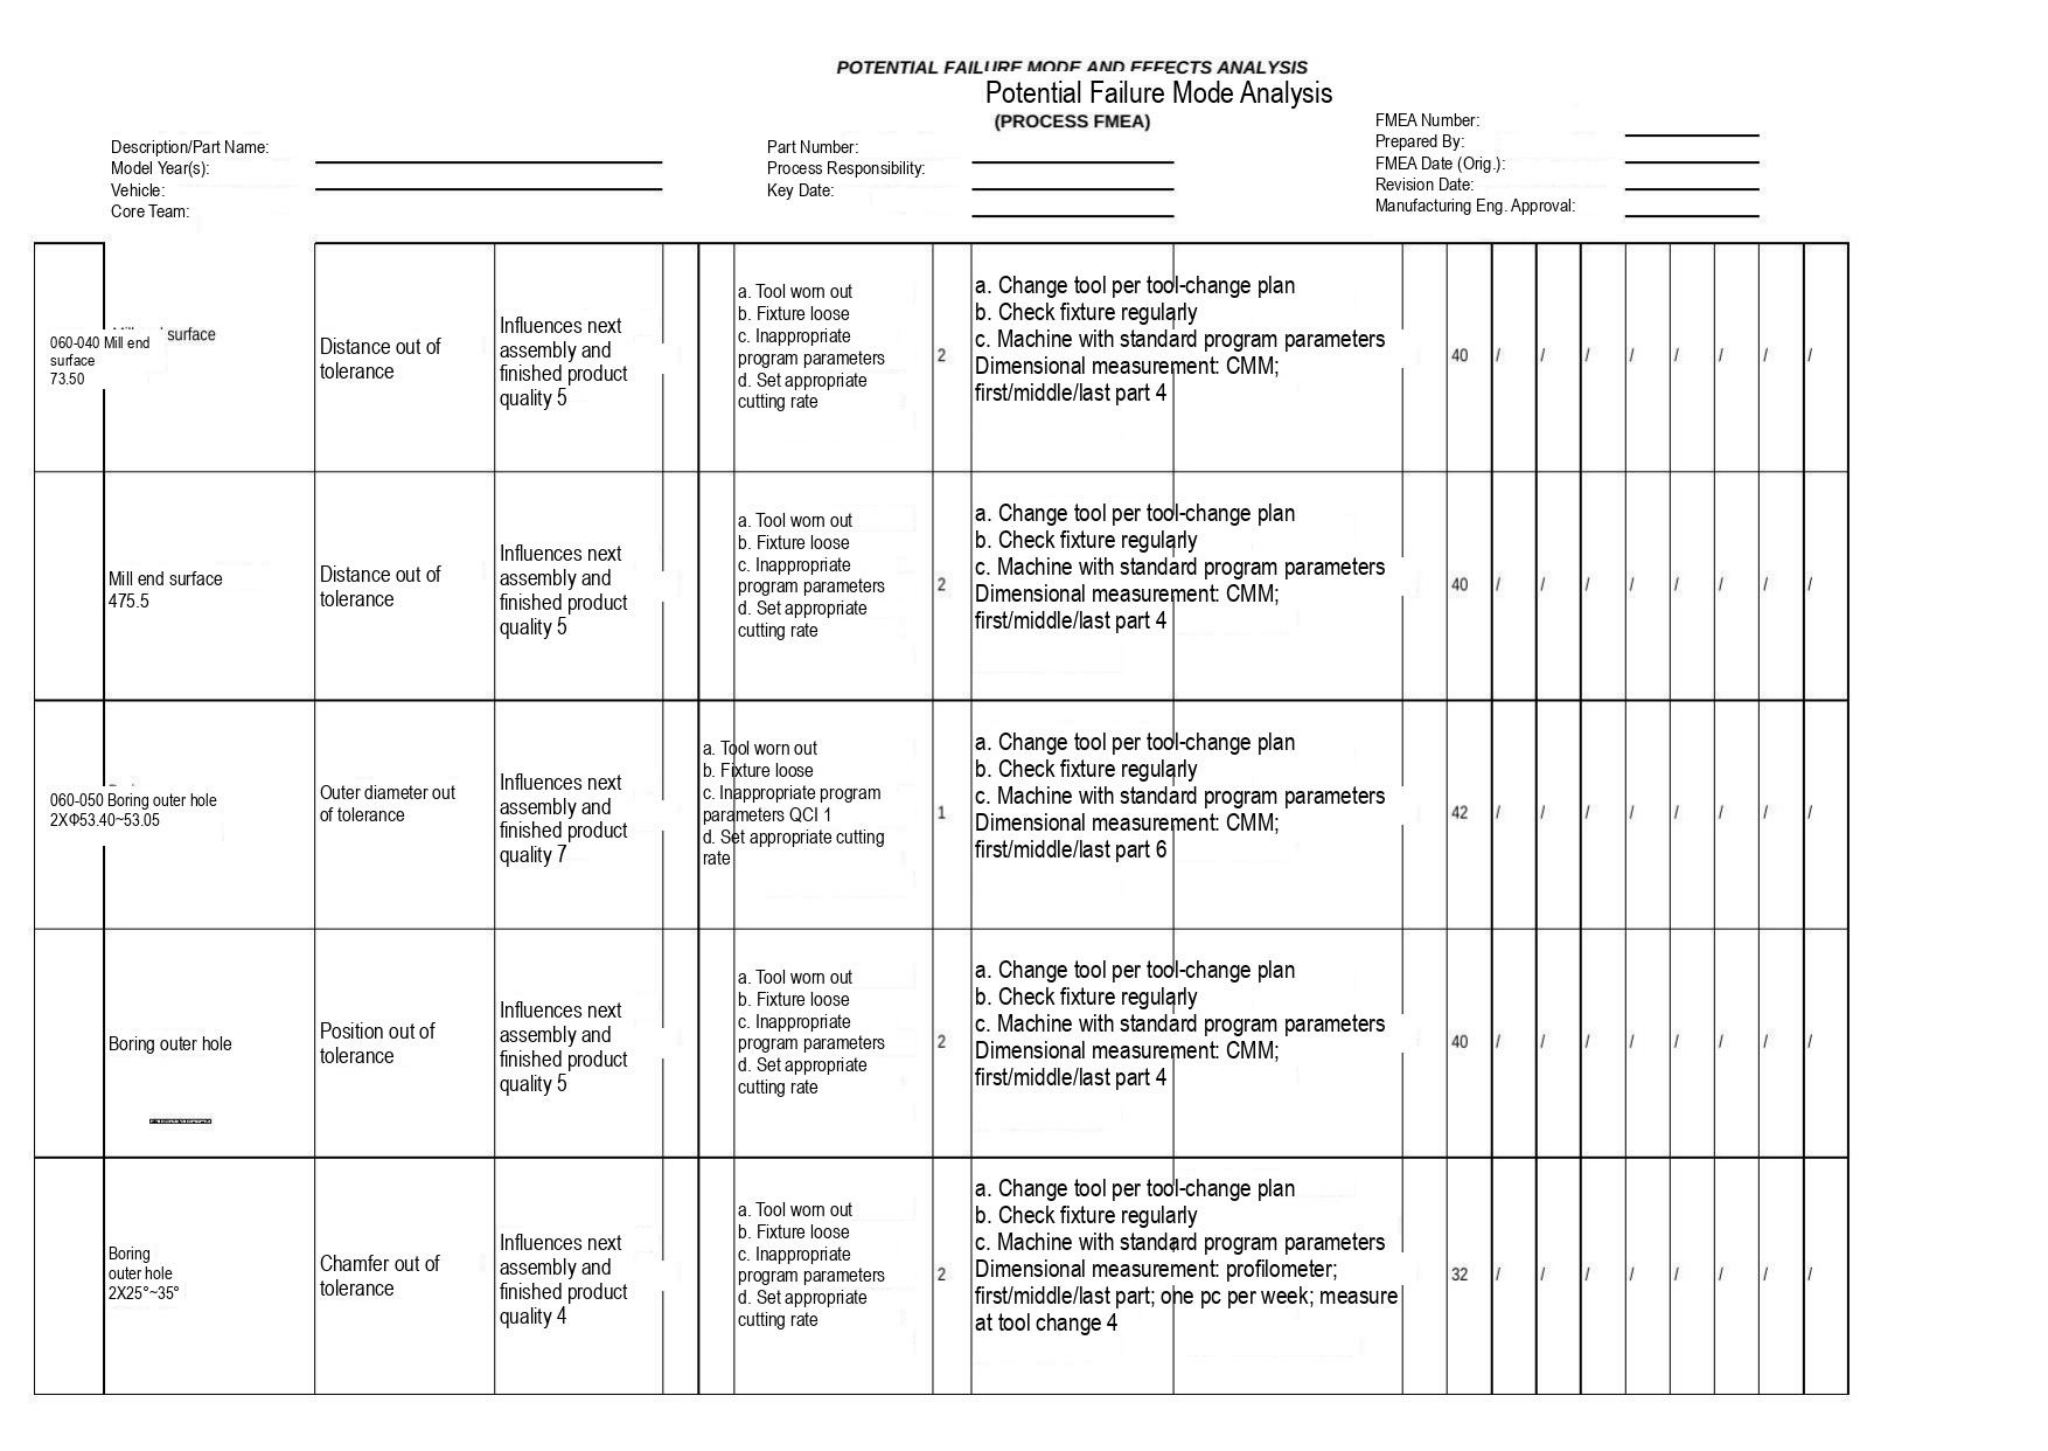**POTENTIAL FAILURE MODE AND EFFECTS ANALYSIS**

Potential Failure Mode Analysis

**(PROCESS FMEA)**

Description/Part Name:
Model Year(s):
Vehicle:
Core Team:

Part Number:
Process Responsibility:
Key Date:

FMEA Number:
Prepared By:
FMEA Date (Orig.):
Revision Date:
Manufacturing Eng. Approval:

| | | | | | | | | | | | | | | | | | | | |
|---|---|---|---|---|---|---|---|---|---|---|---|---|---|---|---|---|---|---|---|
| 060-040 Mill end surface 73.50 | surface | Distance out of tolerance | Influences next assembly and finished product quality 5 | | | a. Tool worn out<br>b. Fixture loose<br>c. Inappropriate program parameters<br>d. Set appropriate cutting rate | 2 | a. Change tool per tool-change plan<br>b. Check fixture regularly<br>c. Machine with standard program parameters<br>Dimensional measurement: CMM; first/middle/last part 4 | | | 40 | / | / | / | / | / | / | / | / |
| | Mill end surface 475.5 | Distance out of tolerance | Influences next assembly and finished product quality 5 | | | a. Tool worn out<br>b. Fixture loose<br>c. Inappropriate program parameters<br>d. Set appropriate cutting rate | 2 | a. Change tool per tool-change plan<br>b. Check fixture regularly<br>c. Machine with standard program parameters<br>Dimensional measurement: CMM; first/middle/last part 4 | | | 40 | / | / | / | / | / | / | / | / |
| 060-050 Boring outer hole 2XΦ53.40~53.05 | | Outer diameter out of tolerance | Influences next assembly and finished product quality 7 | | a. Tool worn out<br>b. Fixture loose<br>c. Inappropriate program parameters QCI 1<br>d. Set appropriate cutting rate | | 1 | a. Change tool per tool-change plan<br>b. Check fixture regularly<br>c. Machine with standard program parameters<br>Dimensional measurement: CMM; first/middle/last part 6 | | | 42 | / | / | / | / | / | / | / | / |
| | Boring outer hole | Position out of tolerance | Influences next assembly and finished product quality 5 | | | a. Tool worn out<br>b. Fixture loose<br>c. Inappropriate program parameters<br>d. Set appropriate cutting rate | 2 | a. Change tool per tool-change plan<br>b. Check fixture regularly<br>c. Machine with standard program parameters<br>Dimensional measurement: CMM; first/middle/last part 4 | | | 40 | / | / | / | / | / | / | / | / |
| | Boring outer hole 2X25°~35° | Chamfer out of tolerance | Influences next assembly and finished product quality 4 | | | a. Tool worn out<br>b. Fixture loose<br>c. Inappropriate program parameters<br>d. Set appropriate cutting rate | 2 | a. Change tool per tool-change plan<br>b. Check fixture regularly<br>c. Machine with standard program parameters<br>Dimensional measurement: profilometer; first/middle/last part; one pc per week; measure at tool change 4 | | | 32 | / | / | / | / | / | / | / | / |
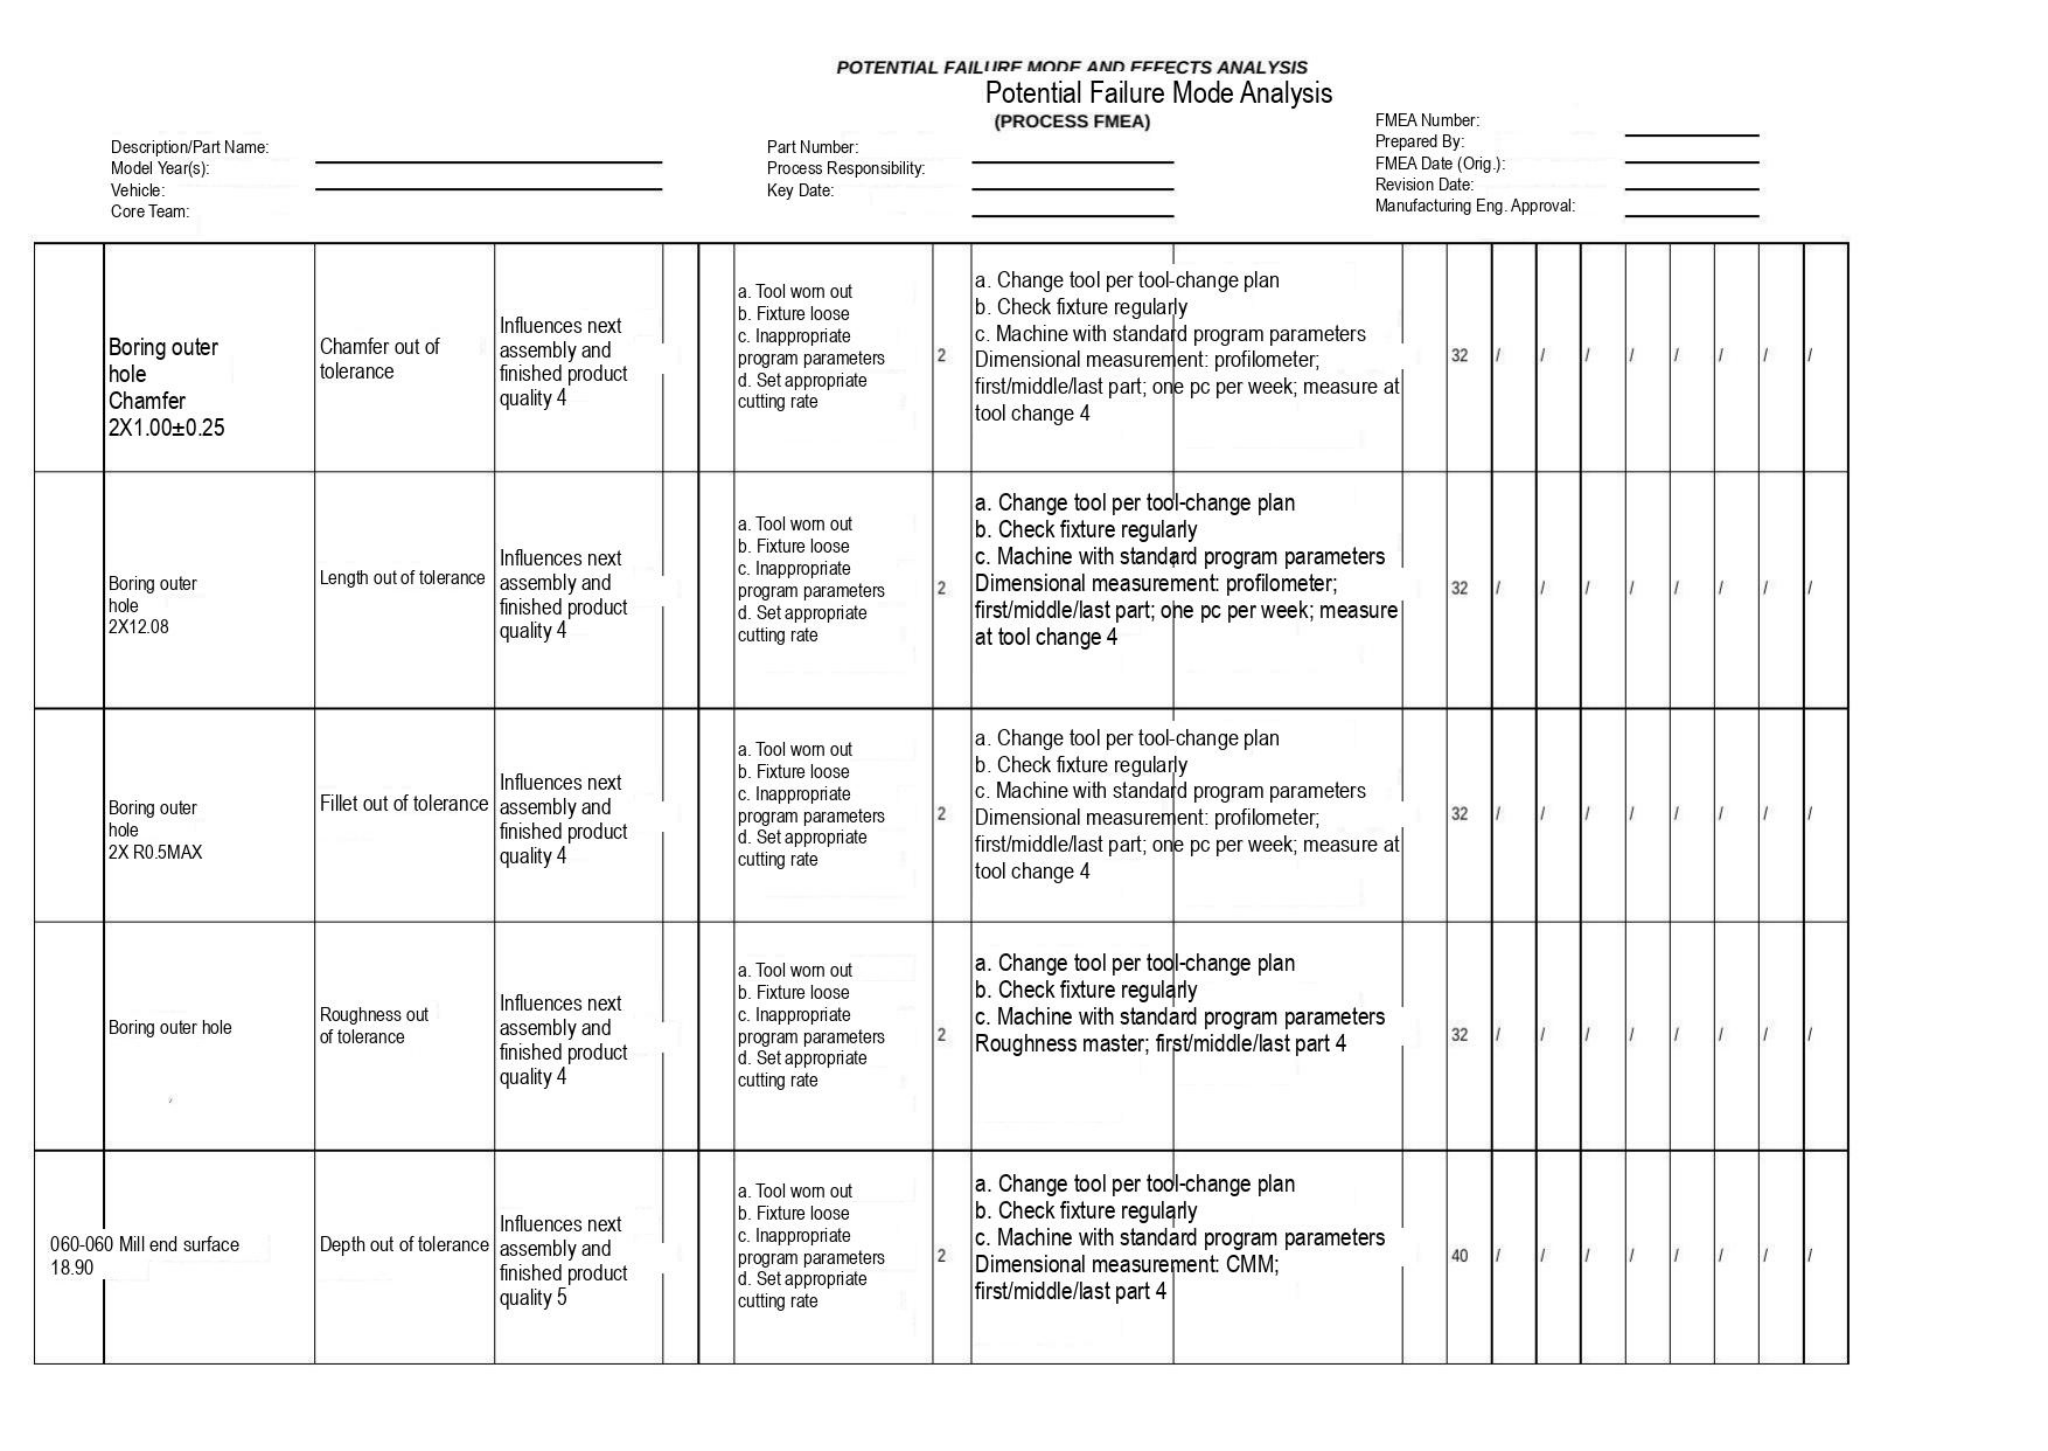POTENTIAL FAILURE MODE AND EFFECTS ANALYSIS

Potential Failure Mode Analysis

(PROCESS FMEA)

Description/Part Name:
Model Year(s):
Vehicle:
Core Team:

Part Number:
Process Responsibility:
Key Date:

FMEA Number:
Prepared By:
FMEA Date (Orig.):
Revision Date:
Manufacturing Eng. Approval:

| | | | | | | | | | | | | | | | | | | |
|---|---|---|---|---|---|---|---|---|---|---|---|---|---|---|---|---|---|---|
| | Boring outer hole Chamfer 2X1.00±0.25 | Chamfer out of tolerance | Influences next assembly and finished product quality 4 | | | a. Tool worn out b. Fixture loose c. Inappropriate program parameters d. Set appropriate cutting rate | 2 | a. Change tool per tool-change plan b. Check fixture regularly c. Machine with standard program parameters Dimensional measurement: profilometer; first/middle/last part; one pc per week; measure at tool change 4 | | 32 | / | / | / | / | / | / | / | / |
| | Boring outer hole 2X12.08 | Length out of tolerance | Influences next assembly and finished product quality 4 | | | a. Tool worn out b. Fixture loose c. Inappropriate program parameters d. Set appropriate cutting rate | 2 | a. Change tool per tool-change plan b. Check fixture regularly c. Machine with standard program parameters Dimensional measurement: profilometer; first/middle/last part; one pc per week; measure at tool change 4 | | 32 | / | / | / | / | / | / | / | / |
| | Boring outer hole 2X R0.5MAX | Fillet out of tolerance | Influences next assembly and finished product quality 4 | | | a. Tool worn out b. Fixture loose c. Inappropriate program parameters d. Set appropriate cutting rate | 2 | a. Change tool per tool-change plan b. Check fixture regularly c. Machine with standard program parameters Dimensional measurement: profilometer; first/middle/last part; one pc per week; measure at tool change 4 | | 32 | / | / | / | / | / | / | / | / |
| | Boring outer hole | Roughness out of tolerance | Influences next assembly and finished product quality 4 | | | a. Tool worn out b. Fixture loose c. Inappropriate program parameters d. Set appropriate cutting rate | 2 | a. Change tool per tool-change plan b. Check fixture regularly c. Machine with standard program parameters Roughness master; first/middle/last part 4 | | 32 | / | / | / | / | / | / | / | / |
| 060-060 Mill end surface 18.90 | | Depth out of tolerance | Influences next assembly and finished product quality 5 | | | a. Tool worn out b. Fixture loose c. Inappropriate program parameters d. Set appropriate cutting rate | 2 | a. Change tool per tool-change plan b. Check fixture regularly c. Machine with standard program parameters Dimensional measurement: CMM; first/middle/last part 4 | | 40 | / | / | / | / | / | / | / | / |
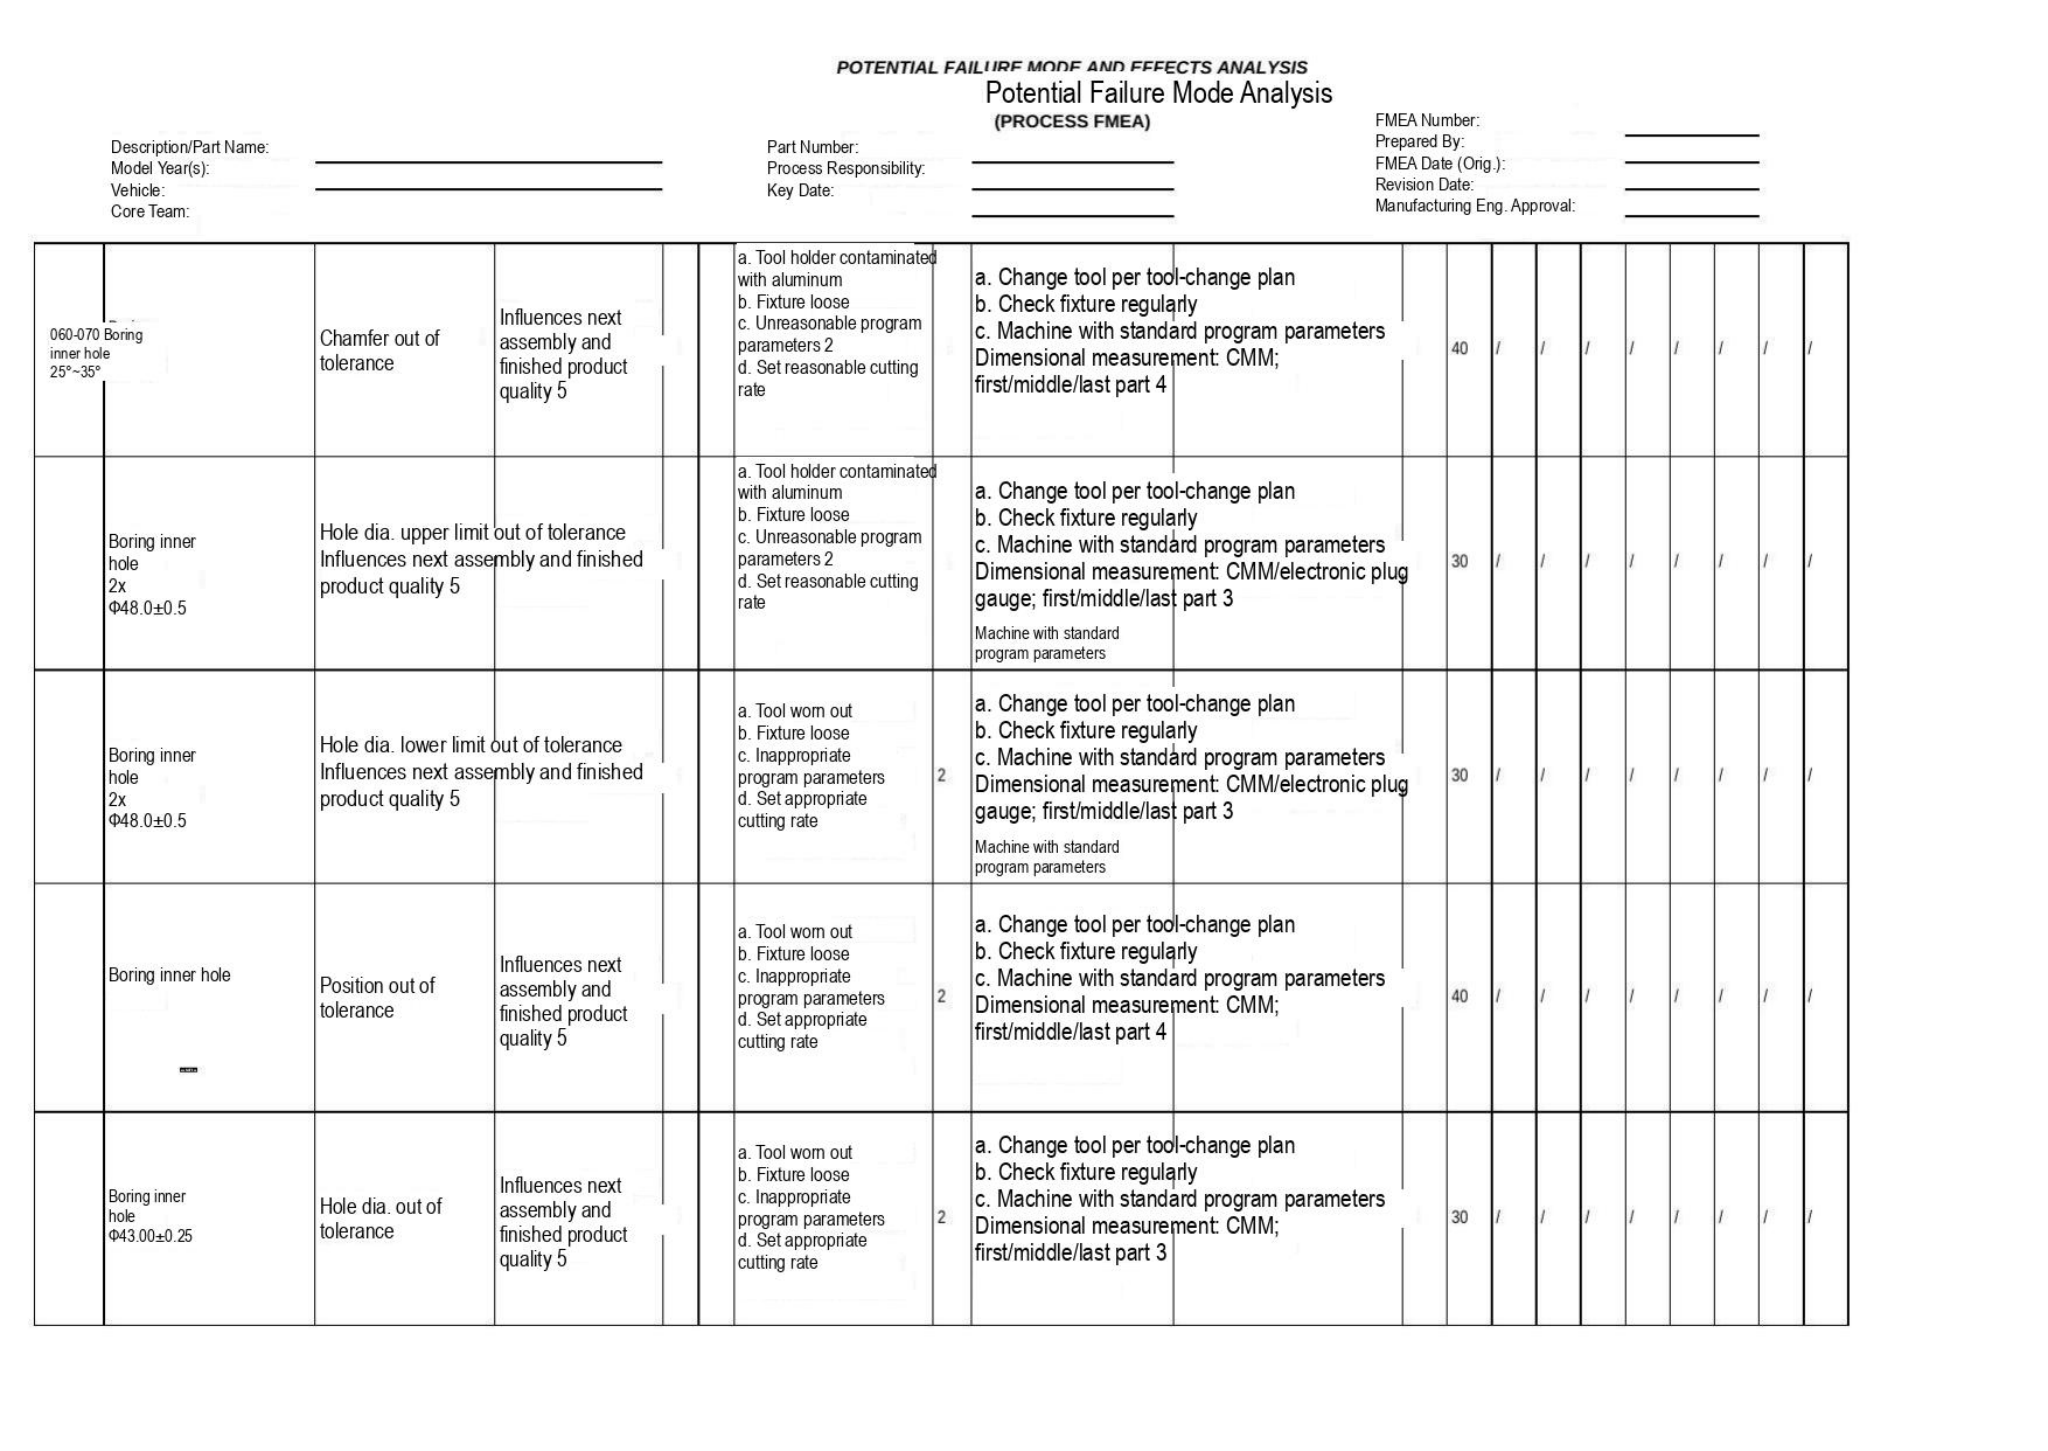**POTENTIAL FAILURE MODE AND EFFECTS ANALYSIS**
Potential Failure Mode Analysis
**(PROCESS FMEA)**

Description/Part Name:
Model Year(s):
Vehicle:
Core Team:

Part Number:
Process Responsibility:
Key Date:

FMEA Number:
Prepared By:
FMEA Date (Orig.):
Revision Date:
Manufacturing Eng. Approval:

| | | | | | | | | | | | | | | | | | | |
|---|---|---|---|---|---|---|---|---|---|---|---|---|---|---|---|---|---|---|
| 060-070 Boring inner hole 25°~35° | | Chamfer out of tolerance | Influences next assembly and finished product quality 5 | | | a. Tool holder contaminated with aluminum<br>b. Fixture loose<br>c. Unreasonable program parameters 2<br>d. Set reasonable cutting rate | | a. Change tool per tool-change plan<br>b. Check fixture regularly<br>c. Machine with standard program parameters<br>Dimensional measurement: CMM; first/middle/last part 4 | | 40 | / | / | / | / | / | / | / | / |
| | Boring inner hole<br>2x<br>Φ48.0±0.5 | Hole dia. upper limit out of tolerance Influences next assembly and finished product quality 5 | | | | a. Tool holder contaminated with aluminum<br>b. Fixture loose<br>c. Unreasonable program parameters 2<br>d. Set reasonable cutting rate | | a. Change tool per tool-change plan<br>b. Check fixture regularly<br>c. Machine with standard program parameters<br>Dimensional measurement: CMM/electronic plug gauge; first/middle/last part 3<br>Machine with standard program parameters | | 30 | / | / | / | / | / | / | / | / |
| | Boring inner hole<br>2x<br>Φ48.0±0.5 | Hole dia. lower limit out of tolerance Influences next assembly and finished product quality 5 | | | | a. Tool worn out<br>b. Fixture loose<br>c. Inappropriate program parameters<br>d. Set appropriate cutting rate | 2 | a. Change tool per tool-change plan<br>b. Check fixture regularly<br>c. Machine with standard program parameters<br>Dimensional measurement: CMM/electronic plug gauge; first/middle/last part 3<br>Machine with standard program parameters | | 30 | / | / | / | / | / | / | / | / |
| | Boring inner hole | Position out of tolerance | Influences next assembly and finished product quality 5 | | | a. Tool worn out<br>b. Fixture loose<br>c. Inappropriate program parameters<br>d. Set appropriate cutting rate | 2 | a. Change tool per tool-change plan<br>b. Check fixture regularly<br>c. Machine with standard program parameters<br>Dimensional measurement: CMM; first/middle/last part 4 | | 40 | / | / | / | / | / | / | / | / |
| | Boring inner hole<br>Φ43.00±0.25 | Hole dia. out of tolerance | Influences next assembly and finished product quality 5 | | | a. Tool worn out<br>b. Fixture loose<br>c. Inappropriate program parameters<br>d. Set appropriate cutting rate | 2 | a. Change tool per tool-change plan<br>b. Check fixture regularly<br>c. Machine with standard program parameters<br>Dimensional measurement: CMM; first/middle/last part 3 | | 30 | / | / | / | / | / | / | / | / |
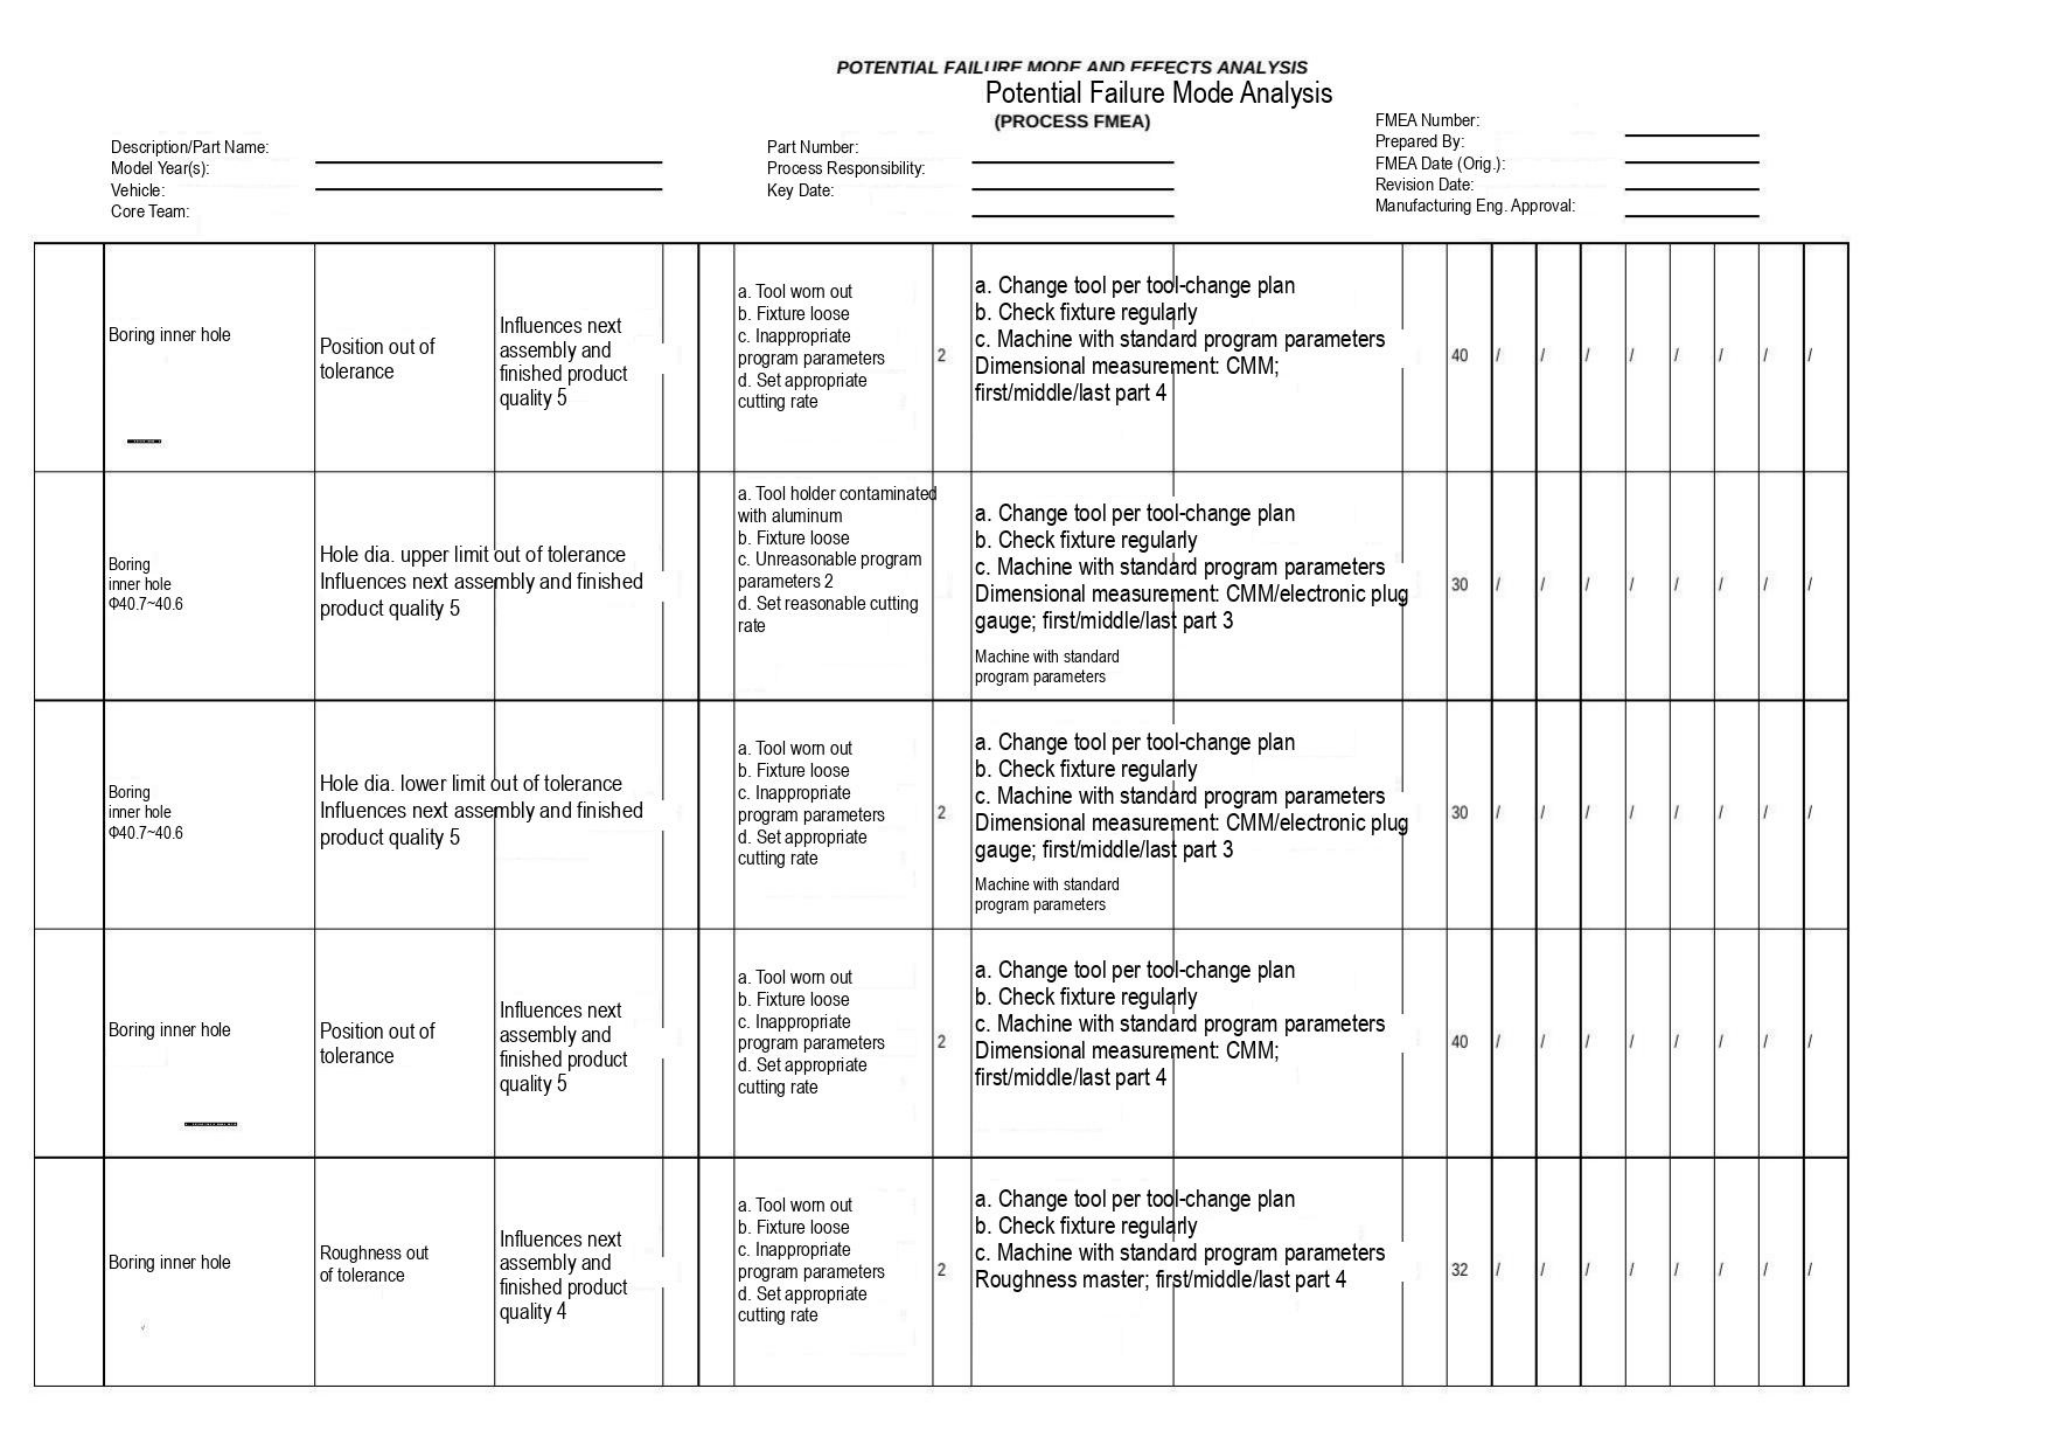**POTENTIAL FAILURE MODE AND EFFECTS ANALYSIS**

Potential Failure Mode Analysis

**(PROCESS FMEA)**

Description/Part Name:
Model Year(s):
Vehicle:
Core Team:

Part Number:
Process Responsibility:
Key Date:

FMEA Number:
Prepared By:
FMEA Date (Orig.):
Revision Date:
Manufacturing Eng. Approval:

| | | | | | | | | | | | | | | | | | | |
|---|---|---|---|---|---|---|---|---|---|---|---|---|---|---|---|---|---|---|
| | Boring inner hole | Position out of tolerance | Influences next assembly and finished product quality 5 | | | a. Tool worn out<br>b. Fixture loose<br>c. Inappropriate program parameters<br>d. Set appropriate cutting rate | 2 | a. Change tool per tool-change plan<br>b. Check fixture regularly<br>c. Machine with standard program parameters<br>Dimensional measurement: CMM;<br>first/middle/last part 4 | | 40 | / | / | / | / | / | / | / | / |
| | Boring<br>inner hole<br>Φ40.7~40.6 | Hole dia. upper limit out of tolerance | Influences next assembly and finished product quality 5 | | | a. Tool holder contaminated with aluminum<br>b. Fixture loose<br>c. Unreasonable program parameters 2<br>d. Set reasonable cutting rate | | a. Change tool per tool-change plan<br>b. Check fixture regularly<br>c. Machine with standard program parameters<br>Dimensional measurement: CMM/electronic plug gauge; first/middle/last part 3<br>Machine with standard program parameters | | 30 | / | / | / | / | / | / | / | / |
| | Boring<br>inner hole<br>Φ40.7~40.6 | Hole dia. lower limit out of tolerance | Influences next assembly and finished product quality 5 | | | a. Tool worn out<br>b. Fixture loose<br>c. Inappropriate program parameters<br>d. Set appropriate cutting rate | 2 | a. Change tool per tool-change plan<br>b. Check fixture regularly<br>c. Machine with standard program parameters<br>Dimensional measurement: CMM/electronic plug gauge; first/middle/last part 3<br>Machine with standard program parameters | | 30 | / | / | / | / | / | / | / | / |
| | Boring inner hole | Position out of tolerance | Influences next assembly and finished product quality 5 | | | a. Tool worn out<br>b. Fixture loose<br>c. Inappropriate program parameters<br>d. Set appropriate cutting rate | 2 | a. Change tool per tool-change plan<br>b. Check fixture regularly<br>c. Machine with standard program parameters<br>Dimensional measurement: CMM;<br>first/middle/last part 4 | | 40 | / | / | / | / | / | / | / | / |
| | Boring inner hole | Roughness out of tolerance | Influences next assembly and finished product quality 4 | | | a. Tool worn out<br>b. Fixture loose<br>c. Inappropriate program parameters<br>d. Set appropriate cutting rate | 2 | a. Change tool per tool-change plan<br>b. Check fixture regularly<br>c. Machine with standard program parameters<br>Roughness master; first/middle/last part 4 | | 32 | / | / | / | / | / | / | / | / |
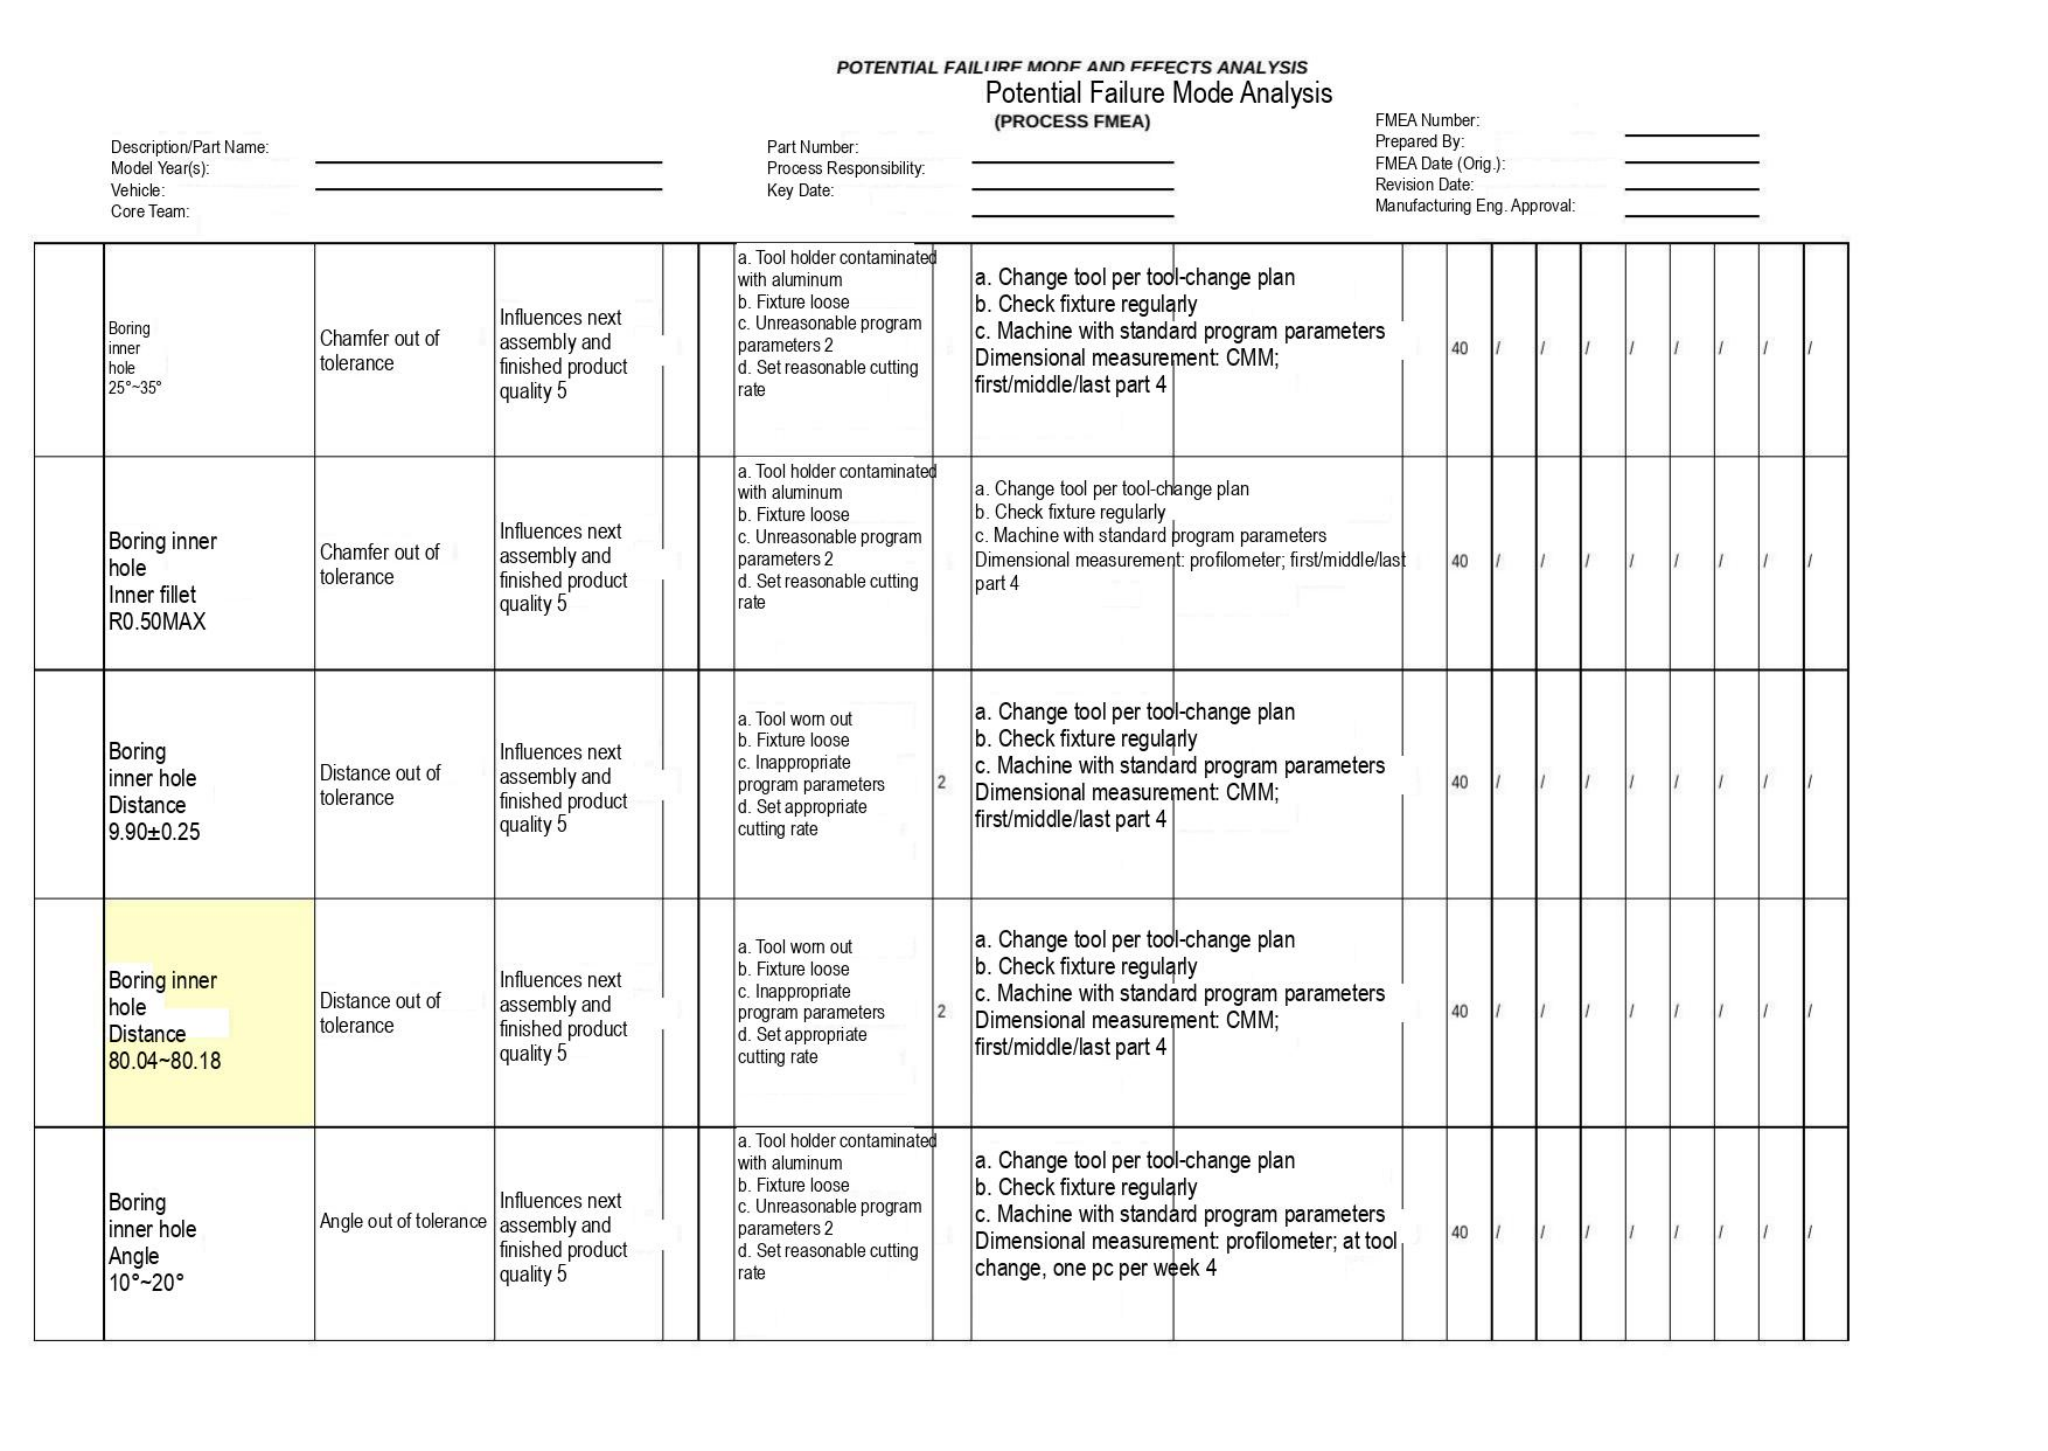**POTENTIAL FAILURE MODE AND EFFECTS ANALYSIS**

Potential Failure Mode Analysis

**(PROCESS FMEA)**

Description/Part Name:
Model Year(s):
Vehicle:
Core Team:

Part Number:
Process Responsibility:
Key Date:

FMEA Number:
Prepared By:
FMEA Date (Orig.):
Revision Date:
Manufacturing Eng. Approval:

| | | | | | | | | | | | | | | | | | | |
|---|---|---|---|---|---|---|---|---|---|---|---|---|---|---|---|---|---|---|
| | Boring inner hole 25°~35° | Chamfer out of tolerance | Influences next assembly and finished product quality 5 | | | a. Tool holder contaminated with aluminum<br>b. Fixture loose<br>c. Unreasonable program parameters 2<br>d. Set reasonable cutting rate | | a. Change tool per tool-change plan<br>b. Check fixture regularly<br>c. Machine with standard program parameters<br>Dimensional measurement: CMM; first/middle/last part 4 | | 40 | / | / | / | / | / | / | / | / |
| | Boring inner hole Inner fillet R0.50MAX | Chamfer out of tolerance | Influences next assembly and finished product quality 5 | | | a. Tool holder contaminated with aluminum<br>b. Fixture loose<br>c. Unreasonable program parameters 2<br>d. Set reasonable cutting rate | | a. Change tool per tool-change plan<br>b. Check fixture regularly<br>c. Machine with standard program parameters<br>Dimensional measurement: profilometer; first/middle/last part 4 | | 40 | / | / | / | / | / | / | / | / |
| | Boring inner hole Distance 9.90±0.25 | Distance out of tolerance | Influences next assembly and finished product quality 5 | | | a. Tool worn out<br>b. Fixture loose<br>c. Inappropriate program parameters<br>d. Set appropriate cutting rate | 2 | a. Change tool per tool-change plan<br>b. Check fixture regularly<br>c. Machine with standard program parameters<br>Dimensional measurement: CMM; first/middle/last part 4 | | 40 | / | / | / | / | / | / | / | / |
| | Boring inner hole Distance 80.04~80.18 | Distance out of tolerance | Influences next assembly and finished product quality 5 | | | a. Tool worn out<br>b. Fixture loose<br>c. Inappropriate program parameters<br>d. Set appropriate cutting rate | 2 | a. Change tool per tool-change plan<br>b. Check fixture regularly<br>c. Machine with standard program parameters<br>Dimensional measurement: CMM; first/middle/last part 4 | | 40 | / | / | / | / | / | / | / | / |
| | Boring inner hole Angle 10°~20° | Angle out of tolerance | Influences next assembly and finished product quality 5 | | | a. Tool holder contaminated with aluminum<br>b. Fixture loose<br>c. Unreasonable program parameters 2<br>d. Set reasonable cutting rate | | a. Change tool per tool-change plan<br>b. Check fixture regularly<br>c. Machine with standard program parameters<br>Dimensional measurement: profilometer; at tool change, one pc per week 4 | | 40 | / | / | / | / | / | / | / | / |
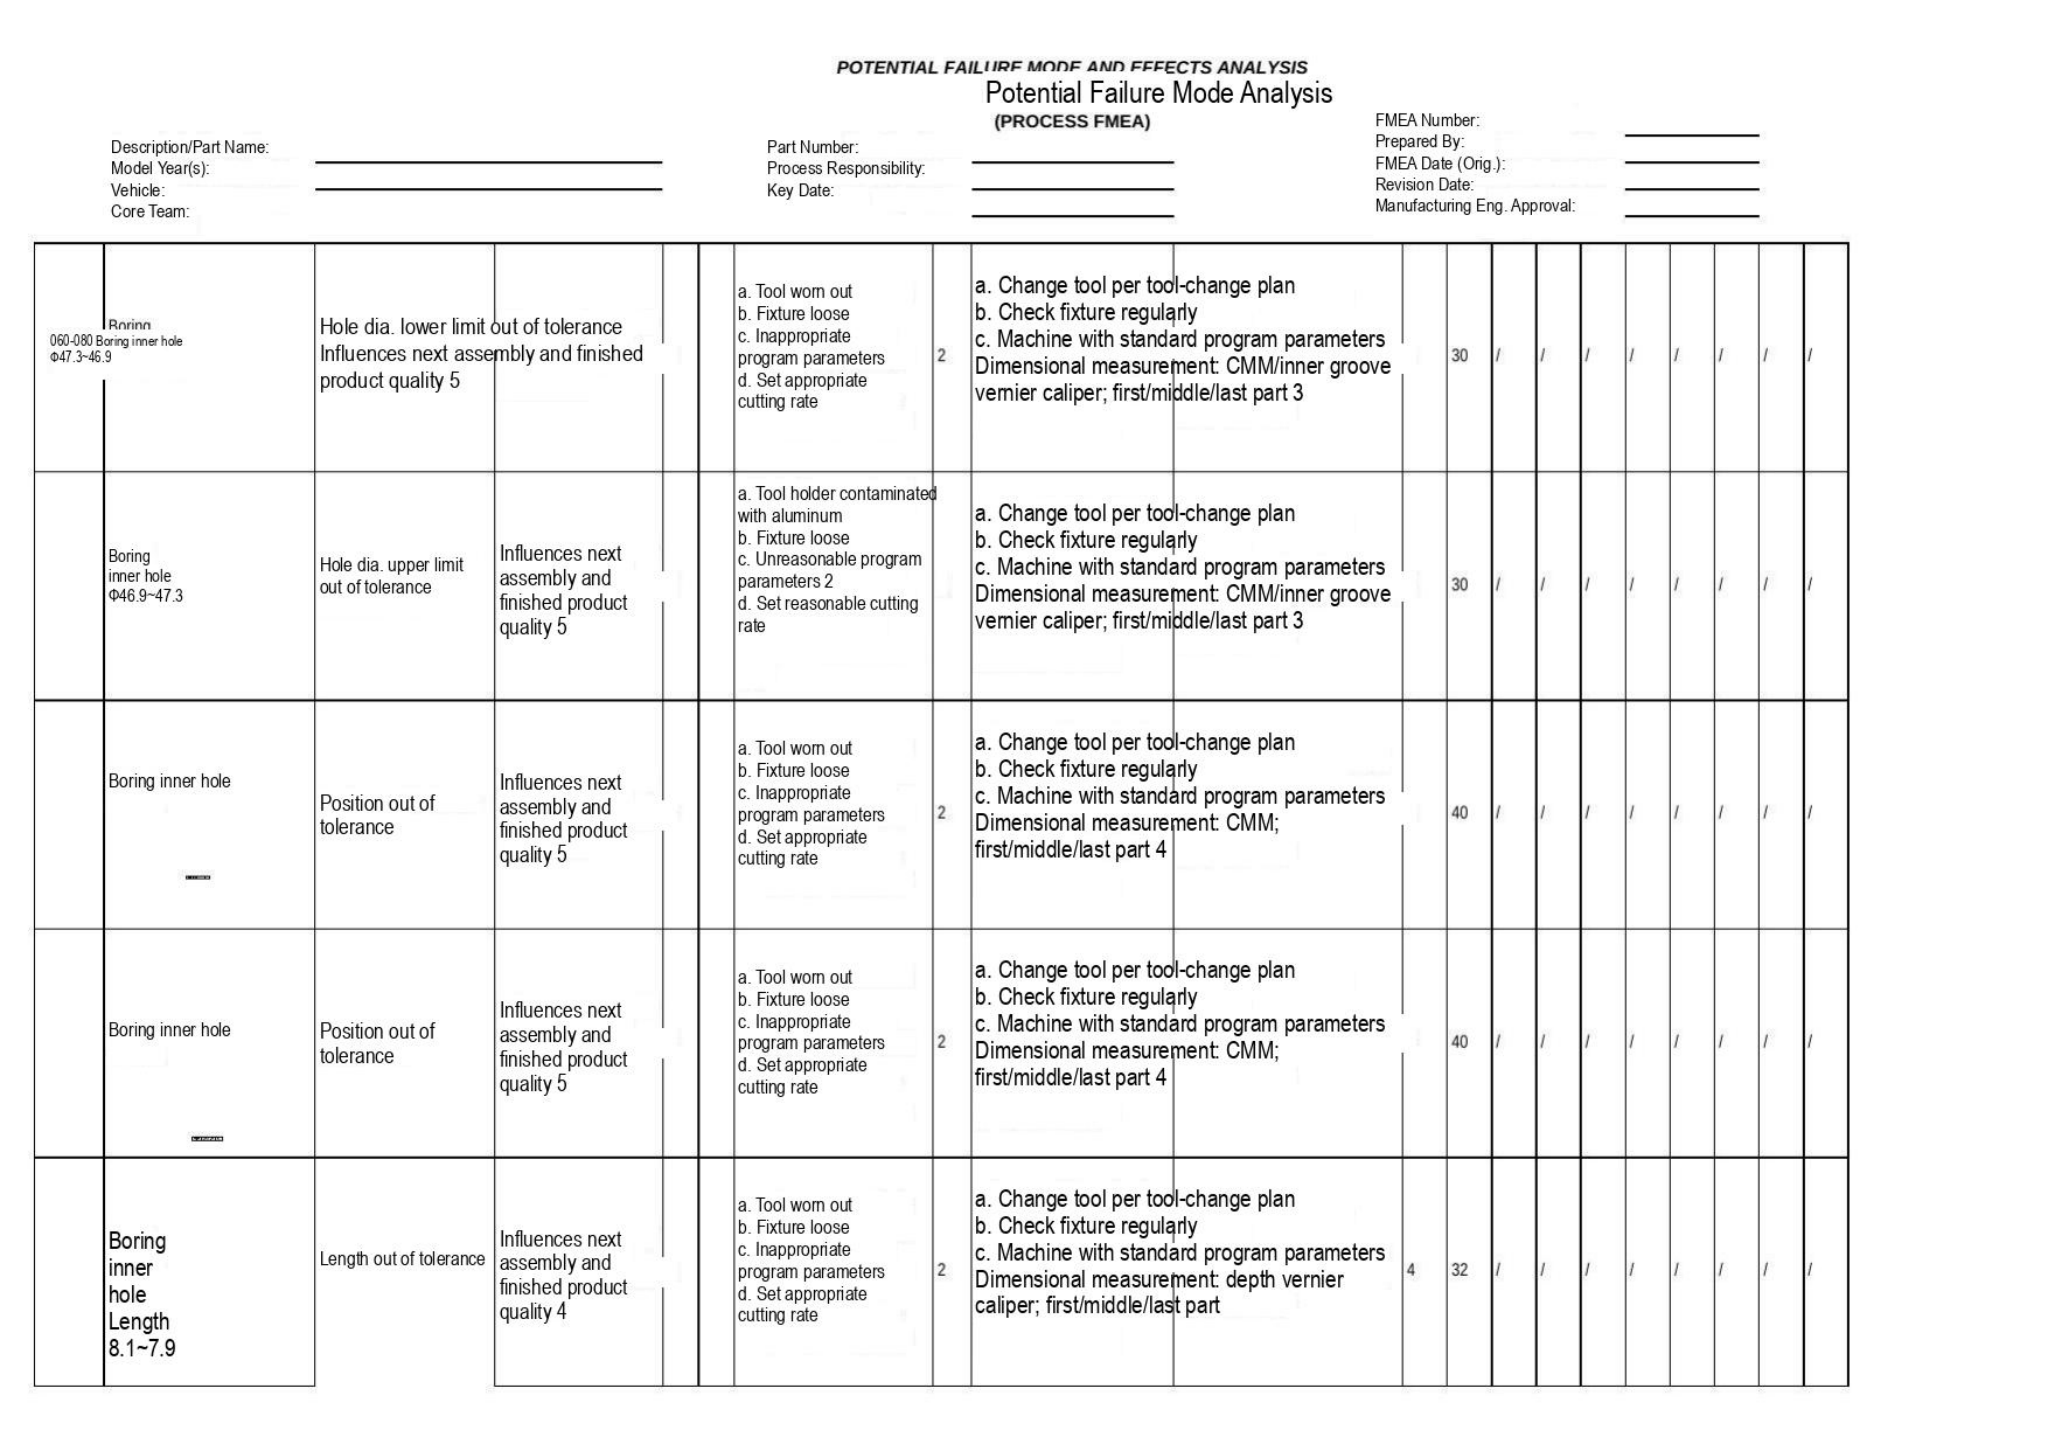**POTENTIAL FAILURE MODE AND EFFECTS ANALYSIS**

Potential Failure Mode Analysis

**(PROCESS FMEA)**

Description/Part Name:
Model Year(s):
Vehicle:
Core Team:

Part Number:
Process Responsibility:
Key Date:

FMEA Number:
Prepared By:
FMEA Date (Orig.):
Revision Date:
Manufacturing Eng. Approval:

| | | | | | | | | | | | | | | | | | | |
|---|---|---|---|---|---|---|---|---|---|---|---|---|---|---|---|---|---|---|
| 060-080 | Boring Boring inner hole Φ47.3~46.9 | Hole dia. lower limit out of tolerance | Influences next assembly and finished product quality 5 | | | a. Tool worn out b. Fixture loose c. Inappropriate program parameters d. Set appropriate cutting rate | 2 | a. Change tool per tool-change plan b. Check fixture regularly c. Machine with standard program parameters Dimensional measurement: CMM/inner groove vernier caliper; first/middle/last part 3 | | 30 | / | / | / | / | / | / | / | / |
| | Boring inner hole Φ46.9~47.3 | Hole dia. upper limit out of tolerance | Influences next assembly and finished product quality 5 | | | a. Tool holder contaminated with aluminum b. Fixture loose c. Unreasonable program parameters 2 d. Set reasonable cutting rate | | a. Change tool per tool-change plan b. Check fixture regularly c. Machine with standard program parameters Dimensional measurement: CMM/inner groove vernier caliper; first/middle/last part 3 | | 30 | / | / | / | / | / | / | / | / |
| | Boring inner hole | Position out of tolerance | Influences next assembly and finished product quality 5 | | | a. Tool worn out b. Fixture loose c. Inappropriate program parameters d. Set appropriate cutting rate | 2 | a. Change tool per tool-change plan b. Check fixture regularly c. Machine with standard program parameters Dimensional measurement: CMM; first/middle/last part 4 | | 40 | / | / | / | / | / | / | / | / |
| | Boring inner hole | Position out of tolerance | Influences next assembly and finished product quality 5 | | | a. Tool worn out b. Fixture loose c. Inappropriate program parameters d. Set appropriate cutting rate | 2 | a. Change tool per tool-change plan b. Check fixture regularly c. Machine with standard program parameters Dimensional measurement: CMM; first/middle/last part 4 | | 40 | / | / | / | / | / | / | / | / |
| | Boring inner hole Length 8.1~7.9 | Length out of tolerance | Influences next assembly and finished product quality 4 | | | a. Tool worn out b. Fixture loose c. Inappropriate program parameters d. Set appropriate cutting rate | 2 | a. Change tool per tool-change plan b. Check fixture regularly c. Machine with standard program parameters Dimensional measurement: depth vernier caliper; first/middle/last part | 4 | 32 | / | / | / | / | / | / | / | / |